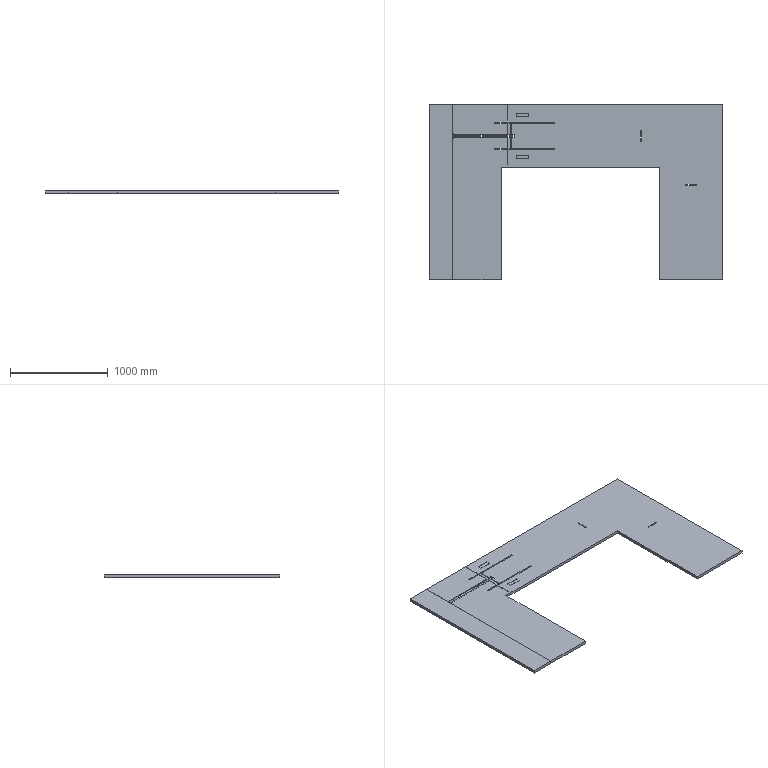Part | STEP file | Table top | 4 solids | 104 faces | box 3010 x 1800 x 30 mm | volume 105133684 mm3 | plane 104